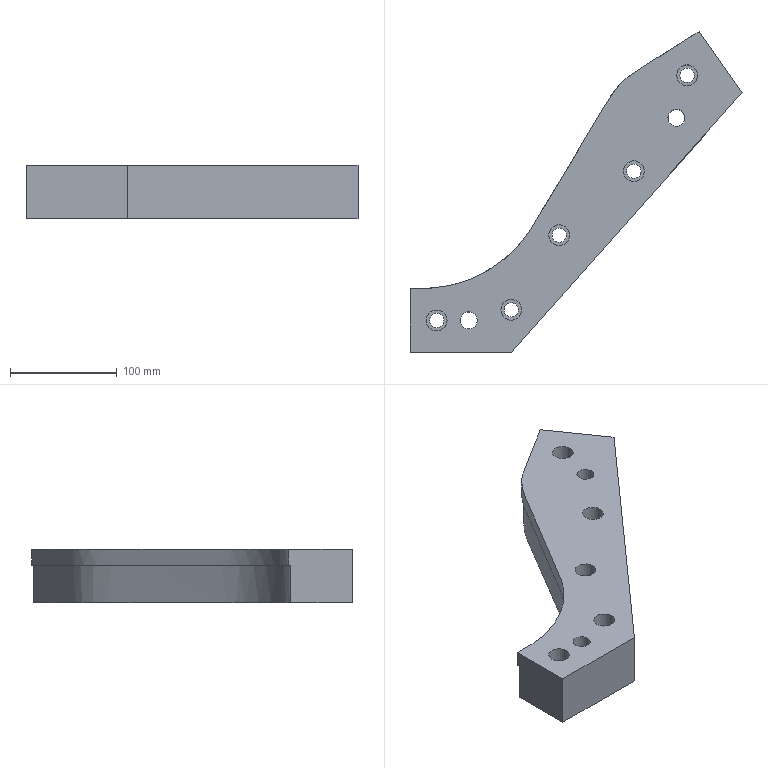Part | NX | features solid 2 | 1 solid | 26 faces | box 311.506 x 301.101 x 50 mm | volume 1333528 mm3 | cylinder 12 | plane 11 | spline 3 | commonest cylinder face diameters 13.5 x5 19.5 x5 16 x2